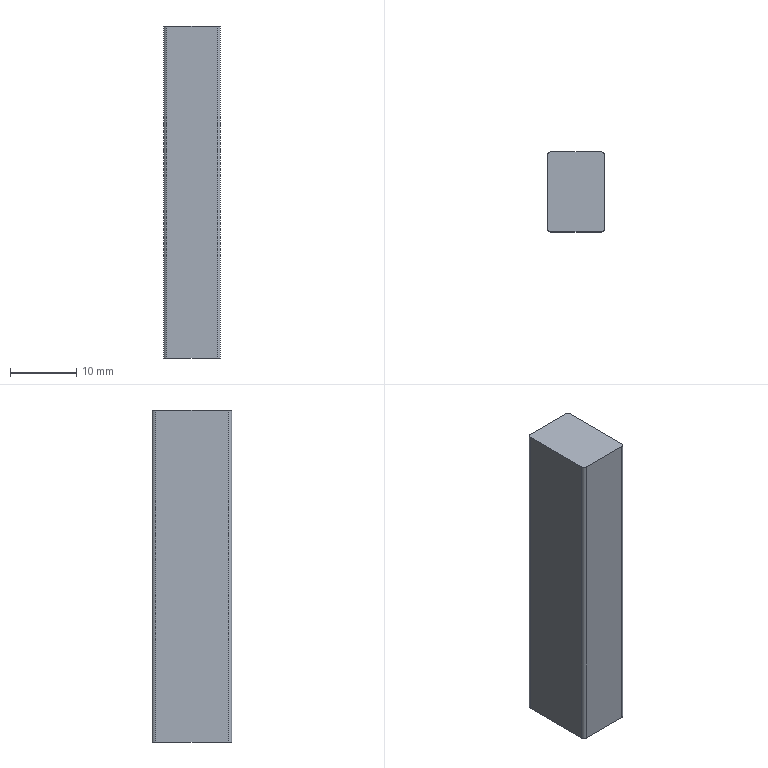Part | NX | features BREP 1 | 1 solid | 10 faces | box 8.547 x 11.991 x 50 mm | volume 5114 mm3 | plane 6 | cylinder 4 | commonest cylinder face diameters 1 x4
STEP:
#1=CARTESIAN_POINT('',(-3.774,5.996,-40.6));
#2=VERTEX_POINT('',#1);
#3=CARTESIAN_POINT('',(-4.274,5.496,-40.6));
#4=VERTEX_POINT('',#3);
#5=CARTESIAN_POINT('',(-3.774,5.496,-40.6));
#6=DIRECTION('',(0.,0.,1.));
#7=DIRECTION('',(1.,0.,0.));
#8=AXIS2_PLACEMENT_3D('',#5,#6,#7);
#9=CIRCLE('',#8,0.5);
#10=EDGE_CURVE('',#2,#4,#9,.T.);
#11=ORIENTED_EDGE('',*,*,#10,.F.);
#12=CARTESIAN_POINT('',(-3.774,5.996,-90.6));
#13=VERTEX_POINT('',#12);
#14=CARTESIAN_POINT('',(-3.774,5.996,-90.6));
#15=DIRECTION('',(0.,0.,1.));
#16=VECTOR('',#15,1000.);
#17=LINE('',#14,#16);
#18=EDGE_CURVE('',#13,#2,#17,.T.);
#19=ORIENTED_EDGE('',*,*,#18,.F.);
#20=CARTESIAN_POINT('',(-4.274,5.496,-90.6));
#21=VERTEX_POINT('',#20);
#22=CARTESIAN_POINT('',(-3.774,5.496,-90.6));
#23=DIRECTION('',(0.,0.,1.));
#24=DIRECTION('',(1.,0.,0.));
#25=AXIS2_PLACEMENT_3D('',#22,#23,#24);
#26=CIRCLE('',#25,0.5);
#27=EDGE_CURVE('',#13,#21,#26,.T.);
#28=ORIENTED_EDGE('',*,*,#27,.T.);
#29=CARTESIAN_POINT('',(-4.274,5.496,-90.6));
#30=DIRECTION('',(0.,0.,1.));
#31=VECTOR('',#30,1000.);
#32=LINE('',#29,#31);
#33=EDGE_CURVE('',#21,#4,#32,.T.);
#34=ORIENTED_EDGE('',*,*,#33,.T.);
#35=EDGE_LOOP('',(#11,#19,#28,#34));
#36=FACE_BOUND('',#35,.T.);
#37=CARTESIAN_POINT('',(-3.774,5.496,-90.6));
#38=DIRECTION('',(0.,0.,1.));
#39=DIRECTION('',(-1.,0.,0.));
#40=AXIS2_PLACEMENT_3D('',#37,#38,#39);
#41=CYLINDRICAL_SURFACE('',#40,0.5);
#42=ADVANCED_FACE('',(#36),#41,.T.);
#43=CARTESIAN_POINT('',(-4.274,-5.496,-40.6));
#44=VERTEX_POINT('',#43);
#45=CARTESIAN_POINT('',(-4.274,-5.496,-40.6));
#46=DIRECTION('',(0.,1.,0.));
#47=VECTOR('',#46,1000.);
#48=LINE('',#45,#47);
#49=EDGE_CURVE('',#44,#4,#48,.T.);
#50=ORIENTED_EDGE('',*,*,#49,.T.);
#51=ORIENTED_EDGE('',*,*,#33,.F.);
#52=CARTESIAN_POINT('',(-4.274,-5.496,-90.6));
#53=VERTEX_POINT('',#52);
#54=CARTESIAN_POINT('',(-4.274,-5.496,-90.6));
#55=DIRECTION('',(0.,1.,0.));
#56=VECTOR('',#55,1000.);
#57=LINE('',#54,#56);
#58=EDGE_CURVE('',#53,#21,#57,.T.);
#59=ORIENTED_EDGE('',*,*,#58,.F.);
#60=CARTESIAN_POINT('',(-4.274,-5.496,-90.6));
#61=DIRECTION('',(0.,0.,1.));
#62=VECTOR('',#61,1000.);
#63=LINE('',#60,#62);
#64=EDGE_CURVE('',#53,#44,#63,.T.);
#65=ORIENTED_EDGE('',*,*,#64,.T.);
#66=EDGE_LOOP('',(#50,#51,#59,#65));
#67=FACE_BOUND('',#66,.T.);
#68=CARTESIAN_POINT('',(-4.274,-5.496,-90.6));
#69=DIRECTION('',(1.,0.,0.));
#70=DIRECTION('',(0.,-1.,0.));
#71=AXIS2_PLACEMENT_3D('',#68,#69,#70);
#72=PLANE('',#71);
#73=ADVANCED_FACE('',(#67),#72,.F.);
#74=CARTESIAN_POINT('',(-3.774,-5.996,-40.6));
#75=VERTEX_POINT('',#74);
#76=CARTESIAN_POINT('',(-3.774,-5.496,-40.6));
#77=DIRECTION('',(0.,0.,1.));
#78=DIRECTION('',(1.,0.,0.));
#79=AXIS2_PLACEMENT_3D('',#76,#77,#78);
#80=CIRCLE('',#79,0.5);
#81=EDGE_CURVE('',#44,#75,#80,.T.);
#82=ORIENTED_EDGE('',*,*,#81,.F.);
#83=ORIENTED_EDGE('',*,*,#64,.F.);
#84=CARTESIAN_POINT('',(-3.774,-5.996,-90.6));
#85=VERTEX_POINT('',#84);
#86=CARTESIAN_POINT('',(-3.774,-5.496,-90.6));
#87=DIRECTION('',(0.,0.,1.));
#88=DIRECTION('',(1.,0.,0.));
#89=AXIS2_PLACEMENT_3D('',#86,#87,#88);
#90=CIRCLE('',#89,0.5);
#91=EDGE_CURVE('',#53,#85,#90,.T.);
#92=ORIENTED_EDGE('',*,*,#91,.T.);
#93=CARTESIAN_POINT('',(-3.774,-5.996,-90.6));
#94=DIRECTION('',(0.,0.,1.));
#95=VECTOR('',#94,1000.);
#96=LINE('',#93,#95);
#97=EDGE_CURVE('',#85,#75,#96,.T.);
#98=ORIENTED_EDGE('',*,*,#97,.T.);
#99=EDGE_LOOP('',(#82,#83,#92,#98));
#100=FACE_BOUND('',#99,.T.);
#101=CARTESIAN_POINT('',(-3.774,-5.496,-90.6));
#102=DIRECTION('',(0.,0.,1.));
#103=DIRECTION('',(-1.,0.,0.));
#104=AXIS2_PLACEMENT_3D('',#101,#102,#103);
#105=CYLINDRICAL_SURFACE('',#104,0.5);
#106=ADVANCED_FACE('',(#100),#105,.T.);
#107=CARTESIAN_POINT('',(3.774,-5.996,-40.6));
#108=VERTEX_POINT('',#107);
#109=CARTESIAN_POINT('',(3.774,-5.996,-40.6));
#110=DIRECTION('',(-1.,0.,0.));
#111=VECTOR('',#110,1000.);
#112=LINE('',#109,#111);
#113=EDGE_CURVE('',#108,#75,#112,.T.);
#114=ORIENTED_EDGE('',*,*,#113,.T.);
#115=ORIENTED_EDGE('',*,*,#97,.F.);
#116=CARTESIAN_POINT('',(3.774,-5.996,-90.6));
#117=VERTEX_POINT('',#116);
#118=CARTESIAN_POINT('',(3.774,-5.996,-90.6));
#119=DIRECTION('',(-1.,0.,0.));
#120=VECTOR('',#119,1000.);
#121=LINE('',#118,#120);
#122=EDGE_CURVE('',#117,#85,#121,.T.);
#123=ORIENTED_EDGE('',*,*,#122,.F.);
#124=CARTESIAN_POINT('',(3.774,-5.996,-90.6));
#125=DIRECTION('',(0.,0.,1.));
#126=VECTOR('',#125,1000.);
#127=LINE('',#124,#126);
#128=EDGE_CURVE('',#117,#108,#127,.T.);
#129=ORIENTED_EDGE('',*,*,#128,.T.);
#130=EDGE_LOOP('',(#114,#115,#123,#129));
#131=FACE_BOUND('',#130,.T.);
#132=CARTESIAN_POINT('',(3.774,-5.996,-90.6));
#133=DIRECTION('',(0.,1.,0.));
#134=DIRECTION('',(0.,0.,-1.));
#135=AXIS2_PLACEMENT_3D('',#132,#133,#134);
#136=PLANE('',#135);
#137=ADVANCED_FACE('',(#131),#136,.F.);
#138=CARTESIAN_POINT('',(4.274,-5.496,-40.6));
#139=VERTEX_POINT('',#138);
#140=CARTESIAN_POINT('',(3.774,-5.496,-40.6));
#141=DIRECTION('',(0.,0.,1.));
#142=DIRECTION('',(1.,0.,0.));
#143=AXIS2_PLACEMENT_3D('',#140,#141,#142);
#144=CIRCLE('',#143,0.5);
#145=EDGE_CURVE('',#108,#139,#144,.T.);
#146=ORIENTED_EDGE('',*,*,#145,.F.);
#147=ORIENTED_EDGE('',*,*,#128,.F.);
#148=CARTESIAN_POINT('',(4.274,-5.496,-90.6));
#149=VERTEX_POINT('',#148);
#150=CARTESIAN_POINT('',(3.774,-5.496,-90.6));
#151=DIRECTION('',(0.,0.,1.));
#152=DIRECTION('',(1.,0.,0.));
#153=AXIS2_PLACEMENT_3D('',#150,#151,#152);
#154=CIRCLE('',#153,0.5);
#155=EDGE_CURVE('',#117,#149,#154,.T.);
#156=ORIENTED_EDGE('',*,*,#155,.T.);
#157=CARTESIAN_POINT('',(4.274,-5.496,-90.6));
#158=DIRECTION('',(0.,0.,1.));
#159=VECTOR('',#158,1000.);
#160=LINE('',#157,#159);
#161=EDGE_CURVE('',#149,#139,#160,.T.);
#162=ORIENTED_EDGE('',*,*,#161,.T.);
#163=EDGE_LOOP('',(#146,#147,#156,#162));
#164=FACE_BOUND('',#163,.T.);
#165=CARTESIAN_POINT('',(3.774,-5.496,-90.6));
#166=DIRECTION('',(0.,0.,1.));
#167=DIRECTION('',(-1.,0.,0.));
#168=AXIS2_PLACEMENT_3D('',#165,#166,#167);
#169=CYLINDRICAL_SURFACE('',#168,0.5);
#170=ADVANCED_FACE('',(#164),#169,.T.);
#171=CARTESIAN_POINT('',(4.274,5.496,-40.6));
#172=VERTEX_POINT('',#171);
#173=CARTESIAN_POINT('',(4.274,5.496,-40.6));
#174=DIRECTION('',(0.,-1.,0.));
#175=VECTOR('',#174,1000.);
#176=LINE('',#173,#175);
#177=EDGE_CURVE('',#172,#139,#176,.T.);
#178=ORIENTED_EDGE('',*,*,#177,.T.);
#179=ORIENTED_EDGE('',*,*,#161,.F.);
#180=CARTESIAN_POINT('',(4.274,5.496,-90.6));
#181=VERTEX_POINT('',#180);
#182=CARTESIAN_POINT('',(4.274,5.496,-90.6));
#183=DIRECTION('',(0.,-1.,0.));
#184=VECTOR('',#183,1000.);
#185=LINE('',#182,#184);
#186=EDGE_CURVE('',#181,#149,#185,.T.);
#187=ORIENTED_EDGE('',*,*,#186,.F.);
#188=CARTESIAN_POINT('',(4.274,5.496,-90.6));
#189=DIRECTION('',(0.,0.,1.));
#190=VECTOR('',#189,1000.);
#191=LINE('',#188,#190);
#192=EDGE_CURVE('',#181,#172,#191,.T.);
#193=ORIENTED_EDGE('',*,*,#192,.T.);
#194=EDGE_LOOP('',(#178,#179,#187,#193));
#195=FACE_BOUND('',#194,.T.);
#196=CARTESIAN_POINT('',(4.274,5.496,-90.6));
#197=DIRECTION('',(-1.,0.,0.));
#198=DIRECTION('',(0.,0.,-1.));
#199=AXIS2_PLACEMENT_3D('',#196,#197,#198);
#200=PLANE('',#199);
#201=ADVANCED_FACE('',(#195),#200,.F.);
#202=CARTESIAN_POINT('',(3.774,5.996,-40.6));
#203=VERTEX_POINT('',#202);
#204=CARTESIAN_POINT('',(3.774,5.496,-40.6));
#205=DIRECTION('',(0.,0.,1.));
#206=DIRECTION('',(1.,0.,0.));
#207=AXIS2_PLACEMENT_3D('',#204,#205,#206);
#208=CIRCLE('',#207,0.5);
#209=EDGE_CURVE('',#172,#203,#208,.T.);
#210=ORIENTED_EDGE('',*,*,#209,.F.);
#211=ORIENTED_EDGE('',*,*,#192,.F.);
#212=CARTESIAN_POINT('',(3.774,5.996,-90.6));
#213=VERTEX_POINT('',#212);
#214=CARTESIAN_POINT('',(3.774,5.496,-90.6));
#215=DIRECTION('',(0.,0.,1.));
#216=DIRECTION('',(1.,0.,0.));
#217=AXIS2_PLACEMENT_3D('',#214,#215,#216);
#218=CIRCLE('',#217,0.5);
#219=EDGE_CURVE('',#181,#213,#218,.T.);
#220=ORIENTED_EDGE('',*,*,#219,.T.);
#221=CARTESIAN_POINT('',(3.774,5.996,-90.6));
#222=DIRECTION('',(0.,0.,1.));
#223=VECTOR('',#222,1000.);
#224=LINE('',#221,#223);
#225=EDGE_CURVE('',#213,#203,#224,.T.);
#226=ORIENTED_EDGE('',*,*,#225,.T.);
#227=EDGE_LOOP('',(#210,#211,#220,#226));
#228=FACE_BOUND('',#227,.T.);
#229=CARTESIAN_POINT('',(3.774,5.496,-90.6));
#230=DIRECTION('',(0.,0.,1.));
#231=DIRECTION('',(-1.,0.,0.));
#232=AXIS2_PLACEMENT_3D('',#229,#230,#231);
#233=CYLINDRICAL_SURFACE('',#232,0.5);
#234=ADVANCED_FACE('',(#228),#233,.T.);
#235=CARTESIAN_POINT('',(-3.774,5.996,-40.6));
#236=DIRECTION('',(1.,0.,0.));
#237=VECTOR('',#236,1000.);
#238=LINE('',#235,#237);
#239=EDGE_CURVE('',#2,#203,#238,.T.);
#240=ORIENTED_EDGE('',*,*,#239,.T.);
#241=ORIENTED_EDGE('',*,*,#225,.F.);
#242=CARTESIAN_POINT('',(-3.774,5.996,-90.6));
#243=DIRECTION('',(1.,0.,0.));
#244=VECTOR('',#243,1000.);
#245=LINE('',#242,#244);
#246=EDGE_CURVE('',#13,#213,#245,.T.);
#247=ORIENTED_EDGE('',*,*,#246,.F.);
#248=ORIENTED_EDGE('',*,*,#18,.T.);
#249=EDGE_LOOP('',(#240,#241,#247,#248));
#250=FACE_BOUND('',#249,.T.);
#251=CARTESIAN_POINT('',(-3.774,5.996,-90.6));
#252=DIRECTION('',(0.,-1.,0.));
#253=DIRECTION('',(0.,0.,1.));
#254=AXIS2_PLACEMENT_3D('',#251,#252,#253);
#255=PLANE('',#254);
#256=ADVANCED_FACE('',(#250),#255,.F.);
#257=ORIENTED_EDGE('',*,*,#27,.F.);
#258=ORIENTED_EDGE('',*,*,#246,.T.);
#259=ORIENTED_EDGE('',*,*,#219,.F.);
#260=ORIENTED_EDGE('',*,*,#186,.T.);
#261=ORIENTED_EDGE('',*,*,#155,.F.);
#262=ORIENTED_EDGE('',*,*,#122,.T.);
#263=ORIENTED_EDGE('',*,*,#91,.F.);
#264=ORIENTED_EDGE('',*,*,#58,.T.);
#265=EDGE_LOOP('',(#257,#258,#259,#260,#261,#262,#263,#264));
#266=FACE_BOUND('',#265,.T.);
#267=CARTESIAN_POINT('',(-3.774,5.496,-90.6));
#268=DIRECTION('',(0.,0.,1.));
#269=DIRECTION('',(-1.,0.,0.));
#270=AXIS2_PLACEMENT_3D('',#267,#268,#269);
#271=PLANE('',#270);
#272=ADVANCED_FACE('',(#266),#271,.F.);
#273=ORIENTED_EDGE('',*,*,#10,.T.);
#274=ORIENTED_EDGE('',*,*,#49,.F.);
#275=ORIENTED_EDGE('',*,*,#81,.T.);
#276=ORIENTED_EDGE('',*,*,#113,.F.);
#277=ORIENTED_EDGE('',*,*,#145,.T.);
#278=ORIENTED_EDGE('',*,*,#177,.F.);
#279=ORIENTED_EDGE('',*,*,#209,.T.);
#280=ORIENTED_EDGE('',*,*,#239,.F.);
#281=EDGE_LOOP('',(#273,#274,#275,#276,#277,#278,#279,#280));
#282=FACE_BOUND('',#281,.T.);
#283=CARTESIAN_POINT('',(-3.774,5.496,-40.6));
#284=DIRECTION('',(0.,0.,1.));
#285=DIRECTION('',(-1.,0.,0.));
#286=AXIS2_PLACEMENT_3D('',#283,#284,#285);
#287=PLANE('',#286);
#288=ADVANCED_FACE('',(#282),#287,.T.);
#289=CLOSED_SHELL('',(#42,#73,#106,#137,#170,#201,#234,#256,#272,#288));
#290=MANIFOLD_SOLID_BREP('',#289);
#291=(LENGTH_UNIT()NAMED_UNIT(*)SI_UNIT(.MILLI.,.METRE.));
#292=UNCERTAINTY_MEASURE_WITH_UNIT(LENGTH_MEASURE(0.00001),#291,'','');
#293=(NAMED_UNIT(*)PLANE_ANGLE_UNIT()SI_UNIT($,.RADIAN.));
#294=(NAMED_UNIT(*)SI_UNIT($,.STERADIAN.)SOLID_ANGLE_UNIT());
#295=(GEOMETRIC_REPRESENTATION_CONTEXT(3)GLOBAL_UNCERTAINTY_ASSIGNED_CONTEXT((#292))GLOBAL_UNIT_ASSIGNED_CONTEXT((#291,#293,#294))REPRESENTATION_CONTEXT('',''));
#296=ADVANCED_BREP_SHAPE_REPRESENTATION('',(#290),#295);